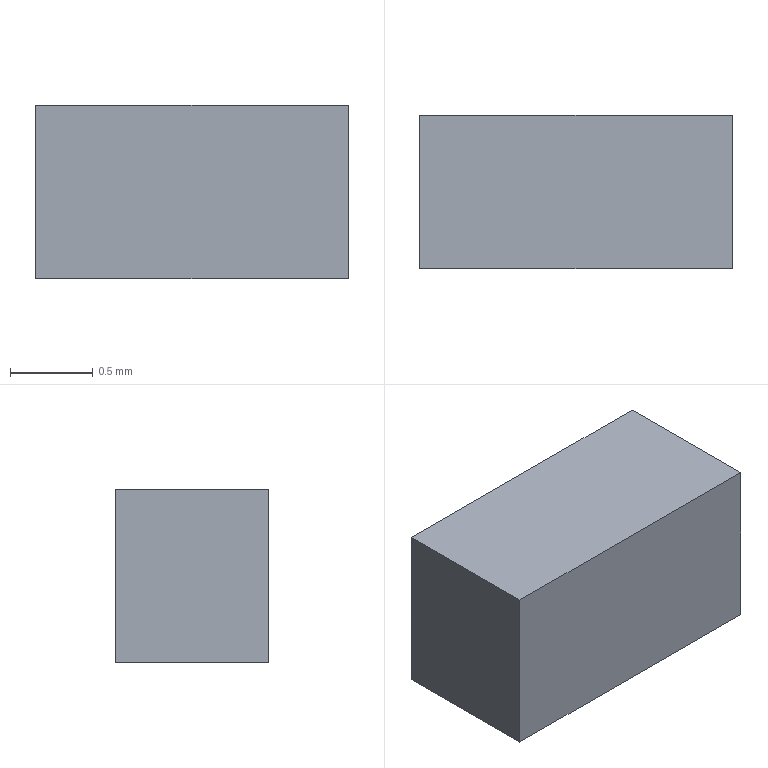Part | Creo | 1 solid | 6 faces | box 1.891 x 0.9288 x 1.053 mm | volume 1.851 mm3 | plane 6
STEP:
#1=CARTESIAN_POINT('',(0.,0.,0.));
#2=DIRECTION('',(0.,0.,1.));
#3=DIRECTION('',(1.,0.,0.));
#4=AXIS2_PLACEMENT_3D('',#1,#2,#3);
#5=CARTESIAN_POINT('',(-0.9404,-0.4484,0.));
#6=VERTEX_POINT('',#5);
#7=CARTESIAN_POINT('',(0.9507,-0.4484,0.));
#8=VERTEX_POINT('',#7);
#9=CARTESIAN_POINT('',(-0.9404,-0.4484,0.));
#10=DIRECTION('',(1.,0.,0.));
#11=VECTOR('',#10,1.891);
#12=LINE('',#9,#11);
#13=EDGE_CURVE('',#6,#8,#12,.T.);
#14=ORIENTED_EDGE('',*,*,#13,.T.);
#15=CARTESIAN_POINT('',(0.9507,0.4804,0.));
#16=VERTEX_POINT('',#15);
#17=CARTESIAN_POINT('',(0.9507,-0.4484,0.));
#18=DIRECTION('',(0.,1.,0.));
#19=VECTOR('',#18,0.9288);
#20=LINE('',#17,#19);
#21=EDGE_CURVE('',#8,#16,#20,.T.);
#22=ORIENTED_EDGE('',*,*,#21,.T.);
#23=CARTESIAN_POINT('',(-0.9404,0.4804,0.));
#24=VERTEX_POINT('',#23);
#25=CARTESIAN_POINT('',(0.9507,0.4804,0.));
#26=DIRECTION('',(-1.,0.,0.));
#27=VECTOR('',#26,1.891);
#28=LINE('',#25,#27);
#29=EDGE_CURVE('',#16,#24,#28,.T.);
#30=ORIENTED_EDGE('',*,*,#29,.T.);
#31=CARTESIAN_POINT('',(-0.9404,0.4804,0.));
#32=DIRECTION('',(0.,-1.,0.));
#33=VECTOR('',#32,0.9288);
#34=LINE('',#31,#33);
#35=EDGE_CURVE('',#24,#6,#34,.T.);
#36=ORIENTED_EDGE('',*,*,#35,.T.);
#37=EDGE_LOOP('',(#14,#22,#30,#36));
#38=FACE_OUTER_BOUND('',#37,.F.);
#39=CARTESIAN_POINT('',(0.,0.,0.));
#40=DIRECTION('',(0.,0.,1.));
#41=DIRECTION('',(1.,0.,0.));
#42=AXIS2_PLACEMENT_3D('',#39,#40,#41);
#43=PLANE('',#42);
#44=ADVANCED_FACE('',(#38),#43,.F.);
#45=ORIENTED_EDGE('',*,*,#13,.F.);
#46=CARTESIAN_POINT('',(-0.9404,-0.4484,1.053));
#47=VERTEX_POINT('',#46);
#48=CARTESIAN_POINT('',(-0.9404,-0.4484,0.));
#49=DIRECTION('',(0.,0.,1.));
#50=VECTOR('',#49,1.053);
#51=LINE('',#48,#50);
#52=EDGE_CURVE('',#6,#47,#51,.T.);
#53=ORIENTED_EDGE('',*,*,#52,.T.);
#54=CARTESIAN_POINT('',(0.9507,-0.4484,1.053));
#55=VERTEX_POINT('',#54);
#56=CARTESIAN_POINT('',(-0.9404,-0.4484,1.053));
#57=DIRECTION('',(1.,0.,0.));
#58=VECTOR('',#57,1.891);
#59=LINE('',#56,#58);
#60=EDGE_CURVE('',#47,#55,#59,.T.);
#61=ORIENTED_EDGE('',*,*,#60,.T.);
#62=CARTESIAN_POINT('',(0.9507,-0.4484,0.));
#63=DIRECTION('',(0.,0.,1.));
#64=VECTOR('',#63,1.053);
#65=LINE('',#62,#64);
#66=EDGE_CURVE('',#8,#55,#65,.T.);
#67=ORIENTED_EDGE('',*,*,#66,.F.);
#68=EDGE_LOOP('',(#45,#53,#61,#67));
#69=FACE_OUTER_BOUND('',#68,.F.);
#70=CARTESIAN_POINT('',(-0.9404,-0.4484,0.));
#71=DIRECTION('',(0.,-1.,0.));
#72=DIRECTION('',(1.,0.,0.));
#73=AXIS2_PLACEMENT_3D('',#70,#71,#72);
#74=PLANE('',#73);
#75=ADVANCED_FACE('',(#69),#74,.T.);
#76=ORIENTED_EDGE('',*,*,#35,.F.);
#77=CARTESIAN_POINT('',(-0.9404,0.4804,1.053));
#78=VERTEX_POINT('',#77);
#79=CARTESIAN_POINT('',(-0.9404,0.4804,0.));
#80=DIRECTION('',(0.,0.,1.));
#81=VECTOR('',#80,1.053);
#82=LINE('',#79,#81);
#83=EDGE_CURVE('',#24,#78,#82,.T.);
#84=ORIENTED_EDGE('',*,*,#83,.T.);
#85=CARTESIAN_POINT('',(-0.9404,0.4804,1.053));
#86=DIRECTION('',(0.,-1.,0.));
#87=VECTOR('',#86,0.9288);
#88=LINE('',#85,#87);
#89=EDGE_CURVE('',#78,#47,#88,.T.);
#90=ORIENTED_EDGE('',*,*,#89,.T.);
#91=ORIENTED_EDGE('',*,*,#52,.F.);
#92=EDGE_LOOP('',(#76,#84,#90,#91));
#93=FACE_OUTER_BOUND('',#92,.F.);
#94=CARTESIAN_POINT('',(-0.9404,0.4804,0.));
#95=DIRECTION('',(-1.,0.,0.));
#96=DIRECTION('',(0.,-1.,0.));
#97=AXIS2_PLACEMENT_3D('',#94,#95,#96);
#98=PLANE('',#97);
#99=ADVANCED_FACE('',(#93),#98,.T.);
#100=ORIENTED_EDGE('',*,*,#29,.F.);
#101=CARTESIAN_POINT('',(0.9507,0.4804,1.053));
#102=VERTEX_POINT('',#101);
#103=CARTESIAN_POINT('',(0.9507,0.4804,0.));
#104=DIRECTION('',(0.,0.,1.));
#105=VECTOR('',#104,1.053);
#106=LINE('',#103,#105);
#107=EDGE_CURVE('',#16,#102,#106,.T.);
#108=ORIENTED_EDGE('',*,*,#107,.T.);
#109=CARTESIAN_POINT('',(0.9507,0.4804,1.053));
#110=DIRECTION('',(-1.,0.,0.));
#111=VECTOR('',#110,1.891);
#112=LINE('',#109,#111);
#113=EDGE_CURVE('',#102,#78,#112,.T.);
#114=ORIENTED_EDGE('',*,*,#113,.T.);
#115=ORIENTED_EDGE('',*,*,#83,.F.);
#116=EDGE_LOOP('',(#100,#108,#114,#115));
#117=FACE_OUTER_BOUND('',#116,.F.);
#118=CARTESIAN_POINT('',(0.9507,0.4804,0.));
#119=DIRECTION('',(0.,1.,0.));
#120=DIRECTION('',(-1.,0.,0.));
#121=AXIS2_PLACEMENT_3D('',#118,#119,#120);
#122=PLANE('',#121);
#123=ADVANCED_FACE('',(#117),#122,.T.);
#124=ORIENTED_EDGE('',*,*,#21,.F.);
#125=ORIENTED_EDGE('',*,*,#66,.T.);
#126=CARTESIAN_POINT('',(0.9507,-0.4484,1.053));
#127=DIRECTION('',(0.,1.,0.));
#128=VECTOR('',#127,0.9288);
#129=LINE('',#126,#128);
#130=EDGE_CURVE('',#55,#102,#129,.T.);
#131=ORIENTED_EDGE('',*,*,#130,.T.);
#132=ORIENTED_EDGE('',*,*,#107,.F.);
#133=EDGE_LOOP('',(#124,#125,#131,#132));
#134=FACE_OUTER_BOUND('',#133,.F.);
#135=CARTESIAN_POINT('',(0.9507,-0.4484,0.));
#136=DIRECTION('',(1.,0.,0.));
#137=DIRECTION('',(0.,1.,0.));
#138=AXIS2_PLACEMENT_3D('',#135,#136,#137);
#139=PLANE('',#138);
#140=ADVANCED_FACE('',(#134),#139,.T.);
#141=ORIENTED_EDGE('',*,*,#60,.F.);
#142=ORIENTED_EDGE('',*,*,#89,.F.);
#143=ORIENTED_EDGE('',*,*,#113,.F.);
#144=ORIENTED_EDGE('',*,*,#130,.F.);
#145=EDGE_LOOP('',(#141,#142,#143,#144));
#146=FACE_OUTER_BOUND('',#145,.F.);
#147=CARTESIAN_POINT('',(0.,0.,1.053));
#148=DIRECTION('',(0.,0.,1.));
#149=DIRECTION('',(1.,0.,0.));
#150=AXIS2_PLACEMENT_3D('',#147,#148,#149);
#151=PLANE('',#150);
#152=ADVANCED_FACE('',(#146),#151,.T.);
#153=CLOSED_SHELL('',(#44,#75,#99,#123,#140,#152));
#154=MANIFOLD_SOLID_BREP('',#153);
#155=(LENGTH_UNIT()NAMED_UNIT(*)SI_UNIT(.MILLI.,.METRE.));
#156=UNCERTAINTY_MEASURE_WITH_UNIT(LENGTH_MEASURE(0.0002356),#155,'','');
#157=(NAMED_UNIT(*)PLANE_ANGLE_UNIT()SI_UNIT($,.RADIAN.));
#158=PLANE_ANGLE_MEASURE_WITH_UNIT(PLANE_ANGLE_MEASURE(0.01745),#157);
#159=(CONVERSION_BASED_UNIT('DEGREE',#158)NAMED_UNIT(*)PLANE_ANGLE_UNIT());
#160=(NAMED_UNIT(*)SI_UNIT($,.STERADIAN.)SOLID_ANGLE_UNIT());
#161=(GEOMETRIC_REPRESENTATION_CONTEXT(3)GLOBAL_UNCERTAINTY_ASSIGNED_CONTEXT((#156))GLOBAL_UNIT_ASSIGNED_CONTEXT((#155,#159,#160))REPRESENTATION_CONTEXT('',''));
#162=ADVANCED_BREP_SHAPE_REPRESENTATION('',(#4,#154),#161);